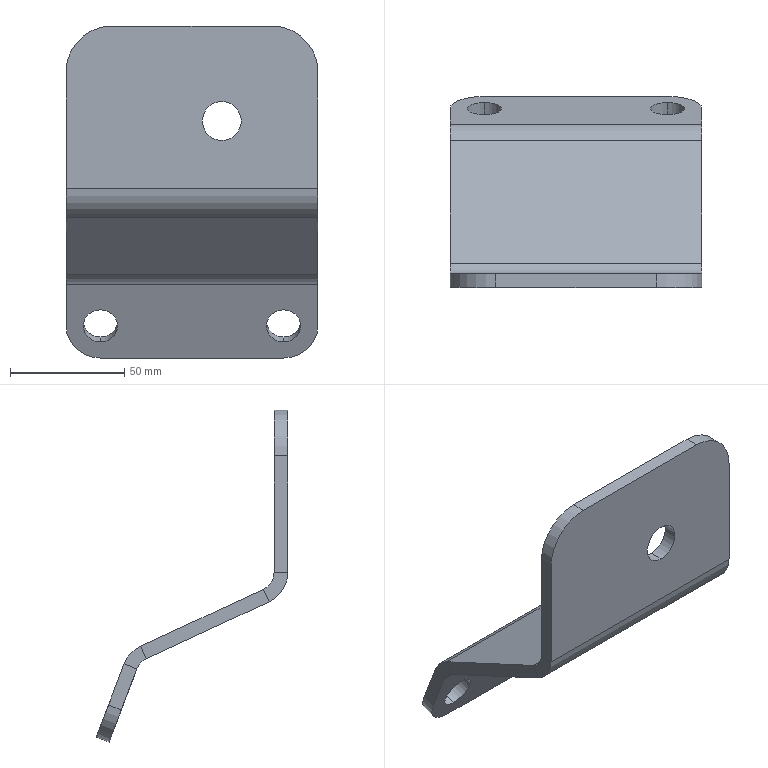Part | SolidWorks | features Fillet 2, ICE 2, FlatPattern 1, SMBaseFlange 1, SheetMetal 1 | 1 solid | 32 faces | box 110 x 83.637 x 145 mm | volume 117261 mm3 | plane 18 | cylinder 14 | commonest cylinder face diameters 15 x4 16 x2 17 x2 28 x2 30 x2 40 x2
STEP:
#1=CARTESIAN_POINT('',(-40.,70.022,-123.973));
#2=VERTEX_POINT('',#1);
#3=CARTESIAN_POINT('',(-40.,75.361,-137.991));
#4=VERTEX_POINT('',#3);
#5=CARTESIAN_POINT('',(-40.,72.691,-130.982));
#6=DIRECTION('',(0.,-0.9345,-0.3559));
#7=DIRECTION('',(0.,-0.3559,0.9345));
#8=AXIS2_PLACEMENT_3D('',#5,#6,#7);
#9=CIRCLE('',#8,7.5);
#10=EDGE_CURVE('',#2,#4,#9,.T.);
#11=ORIENTED_EDGE('',*,*,#10,.T.);
#12=CARTESIAN_POINT('',(-40.,80.968,-135.856));
#13=VERTEX_POINT('',#12);
#14=CARTESIAN_POINT('',(-40.,7.214,-163.946));
#15=DIRECTION('',(0.,0.9345,0.3559));
#16=VECTOR('',#15,1000.);
#17=LINE('',#14,#16);
#18=EDGE_CURVE('',#4,#13,#17,.T.);
#19=ORIENTED_EDGE('',*,*,#18,.T.);
#20=CARTESIAN_POINT('',(-40.,75.629,-121.838));
#21=VERTEX_POINT('',#20);
#22=CARTESIAN_POINT('',(-40.,78.298,-128.847));
#23=DIRECTION('',(0.,0.9345,0.3559));
#24=DIRECTION('',(0.,-0.3559,0.9345));
#25=AXIS2_PLACEMENT_3D('',#22,#23,#24);
#26=CIRCLE('',#25,7.5);
#27=EDGE_CURVE('',#13,#21,#26,.T.);
#28=ORIENTED_EDGE('',*,*,#27,.T.);
#29=CARTESIAN_POINT('',(-40.,1.875,-149.928));
#30=DIRECTION('',(0.,0.9345,0.3559));
#31=VECTOR('',#30,1000.);
#32=LINE('',#29,#31);
#33=EDGE_CURVE('',#2,#21,#32,.T.);
#34=ORIENTED_EDGE('',*,*,#33,.F.);
#35=EDGE_LOOP('',(#11,#19,#28,#34));
#36=FACE_OUTER_BOUND('',#35,.T.);
#37=CARTESIAN_POINT('',(-40.,4.545,-156.937));
#38=DIRECTION('',(0.,0.9345,0.3559));
#39=DIRECTION('',(0.,-0.3559,0.9345));
#40=AXIS2_PLACEMENT_3D('',#37,#38,#39);
#41=CYLINDRICAL_SURFACE('',#40,7.5);
#42=ADVANCED_FACE('',(#36),#41,.F.);
#43=CARTESIAN_POINT('',(40.,70.022,-123.973));
#44=VERTEX_POINT('',#43);
#45=CARTESIAN_POINT('',(40.,75.361,-137.991));
#46=VERTEX_POINT('',#45);
#47=CARTESIAN_POINT('',(40.,72.691,-130.982));
#48=DIRECTION('',(0.,-0.9345,-0.3559));
#49=DIRECTION('',(0.,-0.3559,0.9345));
#50=AXIS2_PLACEMENT_3D('',#47,#48,#49);
#51=CIRCLE('',#50,7.5);
#52=EDGE_CURVE('',#44,#46,#51,.T.);
#53=ORIENTED_EDGE('',*,*,#52,.T.);
#54=CARTESIAN_POINT('',(40.,80.968,-135.856));
#55=VERTEX_POINT('',#54);
#56=CARTESIAN_POINT('',(40.,7.214,-163.946));
#57=DIRECTION('',(0.,0.9345,0.3559));
#58=VECTOR('',#57,1000.);
#59=LINE('',#56,#58);
#60=EDGE_CURVE('',#46,#55,#59,.T.);
#61=ORIENTED_EDGE('',*,*,#60,.T.);
#62=CARTESIAN_POINT('',(40.,75.629,-121.838));
#63=VERTEX_POINT('',#62);
#64=CARTESIAN_POINT('',(40.,78.298,-128.847));
#65=DIRECTION('',(0.,0.9345,0.3559));
#66=DIRECTION('',(0.,-0.3559,0.9345));
#67=AXIS2_PLACEMENT_3D('',#64,#65,#66);
#68=CIRCLE('',#67,7.5);
#69=EDGE_CURVE('',#55,#63,#68,.T.);
#70=ORIENTED_EDGE('',*,*,#69,.T.);
#71=CARTESIAN_POINT('',(40.,1.875,-149.928));
#72=DIRECTION('',(0.,0.9345,0.3559));
#73=VECTOR('',#72,1000.);
#74=LINE('',#71,#73);
#75=EDGE_CURVE('',#44,#63,#74,.T.);
#76=ORIENTED_EDGE('',*,*,#75,.F.);
#77=EDGE_LOOP('',(#53,#61,#70,#76));
#78=FACE_OUTER_BOUND('',#77,.T.);
#79=CARTESIAN_POINT('',(40.,4.545,-156.937));
#80=DIRECTION('',(0.,0.9345,0.3559));
#81=DIRECTION('',(0.,-0.3559,0.9345));
#82=AXIS2_PLACEMENT_3D('',#79,#80,#81);
#83=CYLINDRICAL_SURFACE('',#82,7.5);
#84=ADVANCED_FACE('',(#78),#83,.F.);
#85=CARTESIAN_POINT('',(13.,6.,-33.));
#86=VERTEX_POINT('',#85);
#87=CARTESIAN_POINT('',(13.,6.,-50.));
#88=VERTEX_POINT('',#87);
#89=CARTESIAN_POINT('',(13.,6.,-41.5));
#90=DIRECTION('',(0.,-1.,0.));
#91=DIRECTION('',(0.,0.,1.));
#92=AXIS2_PLACEMENT_3D('',#89,#90,#91);
#93=CIRCLE('',#92,8.5);
#94=EDGE_CURVE('',#86,#88,#93,.T.);
#95=ORIENTED_EDGE('',*,*,#94,.F.);
#96=CARTESIAN_POINT('',(13.,0.,-33.));
#97=VERTEX_POINT('',#96);
#98=CARTESIAN_POINT('',(13.,83.638,-33.));
#99=DIRECTION('',(0.,-1.,0.));
#100=VECTOR('',#99,1000.);
#101=LINE('',#98,#100);
#102=EDGE_CURVE('',#86,#97,#101,.T.);
#103=ORIENTED_EDGE('',*,*,#102,.T.);
#104=CARTESIAN_POINT('',(13.,0.,-50.));
#105=VERTEX_POINT('',#104);
#106=CARTESIAN_POINT('',(13.,0.,-41.5));
#107=DIRECTION('',(0.,-1.,0.));
#108=DIRECTION('',(0.,0.,-1.));
#109=AXIS2_PLACEMENT_3D('',#106,#107,#108);
#110=CIRCLE('',#109,8.5);
#111=EDGE_CURVE('',#97,#105,#110,.T.);
#112=ORIENTED_EDGE('',*,*,#111,.T.);
#113=CARTESIAN_POINT('',(13.,83.638,-50.));
#114=DIRECTION('',(0.,-1.,0.));
#115=VECTOR('',#114,1000.);
#116=LINE('',#113,#115);
#117=EDGE_CURVE('',#88,#105,#116,.T.);
#118=ORIENTED_EDGE('',*,*,#117,.F.);
#119=EDGE_LOOP('',(#95,#103,#112,#118));
#120=FACE_OUTER_BOUND('',#119,.T.);
#121=CARTESIAN_POINT('',(13.,83.638,-41.5));
#122=DIRECTION('',(0.,-1.,0.));
#123=DIRECTION('',(0.,0.,-1.));
#124=AXIS2_PLACEMENT_3D('',#121,#122,#123);
#125=CYLINDRICAL_SURFACE('',#124,8.5);
#126=ADVANCED_FACE('',(#120),#125,.F.);
#127=CARTESIAN_POINT('',(55.,0.,-71.06));
#128=VERTEX_POINT('',#127);
#129=CARTESIAN_POINT('',(55.,6.,-71.06));
#130=VERTEX_POINT('',#129);
#131=CARTESIAN_POINT('',(55.,0.,-71.06));
#132=DIRECTION('',(0.,1.,0.));
#133=VECTOR('',#132,1000.);
#134=LINE('',#131,#133);
#135=EDGE_CURVE('',#128,#130,#134,.T.);
#136=ORIENTED_EDGE('',*,*,#135,.F.);
#137=CARTESIAN_POINT('',(55.,8.111,-83.761));
#138=VERTEX_POINT('',#137);
#139=CARTESIAN_POINT('',(55.,14.,-71.06));
#140=DIRECTION('',(1.,0.,0.));
#141=DIRECTION('',(0.,0.,1.));
#142=AXIS2_PLACEMENT_3D('',#139,#140,#141);
#143=CIRCLE('',#142,14.);
#144=EDGE_CURVE('',#128,#138,#143,.T.);
#145=ORIENTED_EDGE('',*,*,#144,.T.);
#146=CARTESIAN_POINT('',(55.,10.635,-78.317));
#147=VERTEX_POINT('',#146);
#148=CARTESIAN_POINT('',(55.,10.635,-78.317));
#149=DIRECTION('',(0.,-0.4207,-0.9072));
#150=VECTOR('',#149,1000.);
#151=LINE('',#148,#150);
#152=EDGE_CURVE('',#147,#138,#151,.T.);
#153=ORIENTED_EDGE('',*,*,#152,.F.);
#154=CARTESIAN_POINT('',(55.,14.,-71.06));
#155=DIRECTION('',(1.,0.,0.));
#156=DIRECTION('',(0.,0.,-1.));
#157=AXIS2_PLACEMENT_3D('',#154,#155,#156);
#158=CIRCLE('',#157,8.);
#159=EDGE_CURVE('',#130,#147,#158,.T.);
#160=ORIENTED_EDGE('',*,*,#159,.F.);
#161=EDGE_LOOP('',(#136,#145,#153,#160));
#162=FACE_OUTER_BOUND('',#161,.T.);
#163=CARTESIAN_POINT('',(55.,0.,-71.06));
#164=DIRECTION('',(1.,0.,0.));
#165=DIRECTION('',(0.,0.,-1.));
#166=AXIS2_PLACEMENT_3D('',#163,#164,#165);
#167=PLANE('',#166);
#168=ADVANCED_FACE('',(#162),#167,.T.);
#169=CARTESIAN_POINT('',(55.,6.,-20.));
#170=VERTEX_POINT('',#169);
#171=CARTESIAN_POINT('',(55.,6.,0.));
#172=DIRECTION('',(0.,0.,-1.));
#173=VECTOR('',#172,1000.);
#174=LINE('',#171,#173);
#175=EDGE_CURVE('',#170,#130,#174,.T.);
#176=ORIENTED_EDGE('',*,*,#175,.F.);
#177=CARTESIAN_POINT('',(55.,0.,-20.));
#178=VERTEX_POINT('',#177);
#179=CARTESIAN_POINT('',(55.,10.635,-20.));
#180=DIRECTION('',(0.,-1.,0.));
#181=VECTOR('',#180,1000.);
#182=LINE('',#179,#181);
#183=EDGE_CURVE('',#170,#178,#182,.T.);
#184=ORIENTED_EDGE('',*,*,#183,.T.);
#185=CARTESIAN_POINT('',(55.,0.,0.));
#186=DIRECTION('',(0.,0.,-1.));
#187=VECTOR('',#186,1000.);
#188=LINE('',#185,#187);
#189=EDGE_CURVE('',#178,#128,#188,.T.);
#190=ORIENTED_EDGE('',*,*,#189,.T.);
#191=ORIENTED_EDGE('',*,*,#135,.T.);
#192=EDGE_LOOP('',(#176,#184,#190,#191));
#193=FACE_OUTER_BOUND('',#192,.T.);
#194=CARTESIAN_POINT('',(55.,10.635,-78.317));
#195=DIRECTION('',(1.,0.,0.));
#196=DIRECTION('',(0.,0.,-1.));
#197=AXIS2_PLACEMENT_3D('',#194,#195,#196);
#198=PLANE('',#197);
#199=ADVANCED_FACE('',(#193),#198,.T.);
#200=CARTESIAN_POINT('',(-55.,8.111,-83.761));
#201=VERTEX_POINT('',#200);
#202=CARTESIAN_POINT('',(-55.,10.635,-78.317));
#203=VERTEX_POINT('',#202);
#204=CARTESIAN_POINT('',(-55.,8.111,-83.761));
#205=DIRECTION('',(0.,0.4207,0.9072));
#206=VECTOR('',#205,1000.);
#207=LINE('',#204,#206);
#208=EDGE_CURVE('',#201,#203,#207,.T.);
#209=ORIENTED_EDGE('',*,*,#208,.F.);
#210=CARTESIAN_POINT('',(-55.,0.,-71.06));
#211=VERTEX_POINT('',#210);
#212=CARTESIAN_POINT('',(-55.,14.,-71.06));
#213=DIRECTION('',(1.,0.,0.));
#214=DIRECTION('',(0.,0.,1.));
#215=AXIS2_PLACEMENT_3D('',#212,#213,#214);
#216=CIRCLE('',#215,14.);
#217=EDGE_CURVE('',#211,#201,#216,.T.);
#218=ORIENTED_EDGE('',*,*,#217,.F.);
#219=CARTESIAN_POINT('',(-55.,6.,-71.06));
#220=VERTEX_POINT('',#219);
#221=CARTESIAN_POINT('',(-55.,6.,-71.06));
#222=DIRECTION('',(0.,-1.,0.));
#223=VECTOR('',#222,1000.);
#224=LINE('',#221,#223);
#225=EDGE_CURVE('',#220,#211,#224,.T.);
#226=ORIENTED_EDGE('',*,*,#225,.F.);
#227=CARTESIAN_POINT('',(-55.,14.,-71.06));
#228=DIRECTION('',(1.,0.,0.));
#229=DIRECTION('',(0.,0.,-1.));
#230=AXIS2_PLACEMENT_3D('',#227,#228,#229);
#231=CIRCLE('',#230,8.);
#232=EDGE_CURVE('',#220,#203,#231,.T.);
#233=ORIENTED_EDGE('',*,*,#232,.T.);
#234=EDGE_LOOP('',(#209,#218,#226,#233));
#235=FACE_OUTER_BOUND('',#234,.T.);
#236=CARTESIAN_POINT('',(-55.,8.111,-83.761));
#237=DIRECTION('',(-1.,0.,0.));
#238=DIRECTION('',(0.,0.,1.));
#239=AXIS2_PLACEMENT_3D('',#236,#237,#238);
#240=PLANE('',#239);
#241=ADVANCED_FACE('',(#235),#240,.T.);
#242=CARTESIAN_POINT('',(-55.,61.747,-108.631));
#243=VERTEX_POINT('',#242);
#244=CARTESIAN_POINT('',(-55.,0.,-80.));
#245=DIRECTION('',(0.,0.9072,-0.4207));
#246=VECTOR('',#245,1000.);
#247=LINE('',#244,#246);
#248=EDGE_CURVE('',#201,#243,#247,.T.);
#249=ORIENTED_EDGE('',*,*,#248,.F.);
#250=ORIENTED_EDGE('',*,*,#208,.T.);
#251=CARTESIAN_POINT('',(-55.,64.271,-103.188));
#252=VERTEX_POINT('',#251);
#253=CARTESIAN_POINT('',(-55.,2.524,-74.557));
#254=DIRECTION('',(0.,0.9072,-0.4207));
#255=VECTOR('',#254,1000.);
#256=LINE('',#253,#255);
#257=EDGE_CURVE('',#203,#252,#256,.T.);
#258=ORIENTED_EDGE('',*,*,#257,.T.);
#259=CARTESIAN_POINT('',(-55.,64.271,-103.188));
#260=DIRECTION('',(0.,-0.4207,-0.9072));
#261=VECTOR('',#260,1000.);
#262=LINE('',#259,#261);
#263=EDGE_CURVE('',#252,#243,#262,.T.);
#264=ORIENTED_EDGE('',*,*,#263,.T.);
#265=EDGE_LOOP('',(#249,#250,#258,#264));
#266=FACE_OUTER_BOUND('',#265,.T.);
#267=CARTESIAN_POINT('',(-55.,6.,-71.06));
#268=DIRECTION('',(-1.,0.,0.));
#269=DIRECTION('',(0.,0.,1.));
#270=AXIS2_PLACEMENT_3D('',#267,#268,#269);
#271=PLANE('',#270);
#272=ADVANCED_FACE('',(#266),#271,.T.);
#273=CARTESIAN_POINT('',(55.,61.747,-108.631));
#274=VERTEX_POINT('',#273);
#275=CARTESIAN_POINT('',(55.,64.271,-103.188));
#276=VERTEX_POINT('',#275);
#277=CARTESIAN_POINT('',(55.,61.747,-108.631));
#278=DIRECTION('',(0.,0.4207,0.9072));
#279=VECTOR('',#278,1000.);
#280=LINE('',#277,#279);
#281=EDGE_CURVE('',#274,#276,#280,.T.);
#282=ORIENTED_EDGE('',*,*,#281,.F.);
#283=CARTESIAN_POINT('',(55.,65.858,-113.041));
#284=VERTEX_POINT('',#283);
#285=CARTESIAN_POINT('',(55.,58.382,-115.889));
#286=DIRECTION('',(-1.,0.,0.));
#287=DIRECTION('',(0.,0.,-1.));
#288=AXIS2_PLACEMENT_3D('',#285,#286,#287);
#289=CIRCLE('',#288,8.);
#290=EDGE_CURVE('',#274,#284,#289,.T.);
#291=ORIENTED_EDGE('',*,*,#290,.T.);
#292=CARTESIAN_POINT('',(55.,71.465,-110.906));
#293=VERTEX_POINT('',#292);
#294=CARTESIAN_POINT('',(55.,71.465,-110.906));
#295=DIRECTION('',(0.,-0.9345,-0.3559));
#296=VECTOR('',#295,1000.);
#297=LINE('',#294,#296);
#298=EDGE_CURVE('',#293,#284,#297,.T.);
#299=ORIENTED_EDGE('',*,*,#298,.F.);
#300=CARTESIAN_POINT('',(55.,58.382,-115.889));
#301=DIRECTION('',(-1.,0.,0.));
#302=DIRECTION('',(0.,0.,-1.));
#303=AXIS2_PLACEMENT_3D('',#300,#301,#302);
#304=CIRCLE('',#303,14.);
#305=EDGE_CURVE('',#276,#293,#304,.T.);
#306=ORIENTED_EDGE('',*,*,#305,.F.);
#307=EDGE_LOOP('',(#282,#291,#299,#306));
#308=FACE_OUTER_BOUND('',#307,.T.);
#309=CARTESIAN_POINT('',(55.,61.747,-108.631));
#310=DIRECTION('',(1.,0.,0.));
#311=DIRECTION('',(0.,0.,-1.));
#312=AXIS2_PLACEMENT_3D('',#309,#310,#311);
#313=PLANE('',#312);
#314=ADVANCED_FACE('',(#308),#313,.T.);
#315=CARTESIAN_POINT('',(55.,0.,-80.));
#316=DIRECTION('',(0.,0.9072,-0.4207));
#317=VECTOR('',#316,1000.);
#318=LINE('',#315,#317);
#319=EDGE_CURVE('',#138,#274,#318,.T.);
#320=ORIENTED_EDGE('',*,*,#319,.T.);
#321=ORIENTED_EDGE('',*,*,#281,.T.);
#322=CARTESIAN_POINT('',(55.,2.524,-74.557));
#323=DIRECTION('',(0.,0.9072,-0.4207));
#324=VECTOR('',#323,1000.);
#325=LINE('',#322,#324);
#326=EDGE_CURVE('',#147,#276,#325,.T.);
#327=ORIENTED_EDGE('',*,*,#326,.F.);
#328=ORIENTED_EDGE('',*,*,#152,.T.);
#329=EDGE_LOOP('',(#320,#321,#327,#328));
#330=FACE_OUTER_BOUND('',#329,.T.);
#331=CARTESIAN_POINT('',(55.,71.465,-110.906));
#332=DIRECTION('',(1.,0.,0.));
#333=DIRECTION('',(0.,0.,-1.));
#334=AXIS2_PLACEMENT_3D('',#331,#332,#333);
#335=PLANE('',#334);
#336=ADVANCED_FACE('',(#330),#335,.T.);
#337=CARTESIAN_POINT('',(-55.,65.858,-113.041));
#338=VERTEX_POINT('',#337);
#339=CARTESIAN_POINT('',(-55.,71.465,-110.906));
#340=VERTEX_POINT('',#339);
#341=CARTESIAN_POINT('',(-55.,65.858,-113.041));
#342=DIRECTION('',(0.,0.9345,0.3559));
#343=VECTOR('',#342,1000.);
#344=LINE('',#341,#343);
#345=EDGE_CURVE('',#338,#340,#344,.T.);
#346=ORIENTED_EDGE('',*,*,#345,.F.);
#347=CARTESIAN_POINT('',(-55.,58.382,-115.889));
#348=DIRECTION('',(-1.,0.,0.));
#349=DIRECTION('',(0.,0.,-1.));
#350=AXIS2_PLACEMENT_3D('',#347,#348,#349);
#351=CIRCLE('',#350,8.);
#352=EDGE_CURVE('',#243,#338,#351,.T.);
#353=ORIENTED_EDGE('',*,*,#352,.F.);
#354=ORIENTED_EDGE('',*,*,#263,.F.);
#355=CARTESIAN_POINT('',(-55.,58.382,-115.889));
#356=DIRECTION('',(-1.,0.,0.));
#357=DIRECTION('',(0.,0.,-1.));
#358=AXIS2_PLACEMENT_3D('',#355,#356,#357);
#359=CIRCLE('',#358,14.);
#360=EDGE_CURVE('',#252,#340,#359,.T.);
#361=ORIENTED_EDGE('',*,*,#360,.T.);
#362=EDGE_LOOP('',(#346,#353,#354,#361));
#363=FACE_OUTER_BOUND('',#362,.T.);
#364=CARTESIAN_POINT('',(-55.,65.858,-113.041));
#365=DIRECTION('',(-1.,0.,0.));
#366=DIRECTION('',(0.,0.,1.));
#367=AXIS2_PLACEMENT_3D('',#364,#365,#366);
#368=PLANE('',#367);
#369=ADVANCED_FACE('',(#363),#368,.T.);
#370=CARTESIAN_POINT('',(-55.,78.298,-128.847));
#371=VERTEX_POINT('',#370);
#372=CARTESIAN_POINT('',(-55.,70.307,-107.864));
#373=DIRECTION('',(0.,0.3559,-0.9345));
#374=VECTOR('',#373,1000.);
#375=LINE('',#372,#374);
#376=EDGE_CURVE('',#340,#371,#375,.T.);
#377=ORIENTED_EDGE('',*,*,#376,.T.);
#378=CARTESIAN_POINT('',(-55.,72.691,-130.982));
#379=VERTEX_POINT('',#378);
#380=CARTESIAN_POINT('',(-55.,74.583,-130.262));
#381=DIRECTION('',(0.,-0.9345,-0.3559));
#382=VECTOR('',#381,1000.);
#383=LINE('',#380,#382);
#384=EDGE_CURVE('',#371,#379,#383,.T.);
#385=ORIENTED_EDGE('',*,*,#384,.T.);
#386=CARTESIAN_POINT('',(-55.,64.7,-110.));
#387=DIRECTION('',(0.,0.3559,-0.9345));
#388=VECTOR('',#387,1000.);
#389=LINE('',#386,#388);
#390=EDGE_CURVE('',#338,#379,#389,.T.);
#391=ORIENTED_EDGE('',*,*,#390,.F.);
#392=ORIENTED_EDGE('',*,*,#345,.T.);
#393=EDGE_LOOP('',(#377,#385,#391,#392));
#394=FACE_OUTER_BOUND('',#393,.T.);
#395=CARTESIAN_POINT('',(-55.,64.271,-103.188));
#396=DIRECTION('',(-1.,0.,0.));
#397=DIRECTION('',(0.,0.,1.));
#398=AXIS2_PLACEMENT_3D('',#395,#396,#397);
#399=PLANE('',#398);
#400=ADVANCED_FACE('',(#394),#399,.T.);
#401=ORIENTED_EDGE('',*,*,#10,.F.);
#402=CARTESIAN_POINT('',(-40.,72.691,-130.982));
#403=DIRECTION('',(0.,-0.9345,-0.3559));
#404=DIRECTION('',(0.,-0.3559,0.9345));
#405=AXIS2_PLACEMENT_3D('',#402,#403,#404);
#406=CIRCLE('',#405,7.5);
#407=EDGE_CURVE('',#4,#2,#406,.T.);
#408=ORIENTED_EDGE('',*,*,#407,.F.);
#409=EDGE_LOOP('',(#401,#408));
#410=FACE_BOUND('',#409,.T.);
#411=ORIENTED_EDGE('',*,*,#52,.F.);
#412=CARTESIAN_POINT('',(40.,72.691,-130.982));
#413=DIRECTION('',(0.,-0.9345,-0.3559));
#414=DIRECTION('',(0.,-0.3559,0.9345));
#415=AXIS2_PLACEMENT_3D('',#412,#413,#414);
#416=CIRCLE('',#415,7.5);
#417=EDGE_CURVE('',#46,#44,#416,.T.);
#418=ORIENTED_EDGE('',*,*,#417,.F.);
#419=EDGE_LOOP('',(#411,#418));
#420=FACE_BOUND('',#419,.T.);
#421=ORIENTED_EDGE('',*,*,#390,.T.);
#422=CARTESIAN_POINT('',(-40.,78.03,-145.));
#423=VERTEX_POINT('',#422);
#424=CARTESIAN_POINT('',(-40.,72.691,-130.982));
#425=DIRECTION('',(0.,-0.9345,-0.3559));
#426=DIRECTION('',(0.,-0.3559,0.9345));
#427=AXIS2_PLACEMENT_3D('',#424,#425,#426);
#428=CIRCLE('',#427,15.);
#429=EDGE_CURVE('',#379,#423,#428,.T.);
#430=ORIENTED_EDGE('',*,*,#429,.T.);
#431=CARTESIAN_POINT('',(40.,78.03,-145.));
#432=VERTEX_POINT('',#431);
#433=CARTESIAN_POINT('',(55.,78.03,-145.));
#434=DIRECTION('',(-1.,0.,0.));
#435=VECTOR('',#434,1000.);
#436=LINE('',#433,#435);
#437=EDGE_CURVE('',#432,#423,#436,.T.);
#438=ORIENTED_EDGE('',*,*,#437,.F.);
#439=CARTESIAN_POINT('',(55.,72.691,-130.982));
#440=VERTEX_POINT('',#439);
#441=CARTESIAN_POINT('',(40.,72.691,-130.982));
#442=DIRECTION('',(0.,-0.9345,-0.3559));
#443=DIRECTION('',(0.,-0.3559,0.9345));
#444=AXIS2_PLACEMENT_3D('',#441,#442,#443);
#445=CIRCLE('',#444,15.);
#446=EDGE_CURVE('',#432,#440,#445,.T.);
#447=ORIENTED_EDGE('',*,*,#446,.T.);
#448=CARTESIAN_POINT('',(55.,64.7,-110.));
#449=DIRECTION('',(0.,0.3559,-0.9345));
#450=VECTOR('',#449,1000.);
#451=LINE('',#448,#450);
#452=EDGE_CURVE('',#284,#440,#451,.T.);
#453=ORIENTED_EDGE('',*,*,#452,.F.);
#454=CARTESIAN_POINT('',(55.,65.858,-113.041));
#455=DIRECTION('',(-1.,0.,0.));
#456=VECTOR('',#455,1000.);
#457=LINE('',#454,#456);
#458=EDGE_CURVE('',#284,#338,#457,.T.);
#459=ORIENTED_EDGE('',*,*,#458,.T.);
#460=EDGE_LOOP('',(#421,#430,#438,#447,#453,#459));
#461=FACE_OUTER_BOUND('',#460,.T.);
#462=CARTESIAN_POINT('',(55.,64.7,-110.));
#463=DIRECTION('',(0.,0.9345,0.3559));
#464=DIRECTION('',(0.,-0.3559,0.9345));
#465=AXIS2_PLACEMENT_3D('',#462,#463,#464);
#466=PLANE('',#465);
#467=ADVANCED_FACE('',(#410,#420,#461),#466,.F.);
#468=ORIENTED_EDGE('',*,*,#437,.T.);
#469=CARTESIAN_POINT('',(-40.,83.637,-142.864));
#470=VERTEX_POINT('',#469);
#471=CARTESIAN_POINT('',(-40.,83.637,-142.864));
#472=DIRECTION('',(0.,0.9345,0.3559));
#473=VECTOR('',#472,1000.);
#474=LINE('',#471,#473);
#475=EDGE_CURVE('',#423,#470,#474,.T.);
#476=ORIENTED_EDGE('',*,*,#475,.T.);
#477=CARTESIAN_POINT('',(40.,83.637,-142.864));
#478=VERTEX_POINT('',#477);
#479=CARTESIAN_POINT('',(55.,83.637,-142.864));
#480=DIRECTION('',(-1.,0.,0.));
#481=VECTOR('',#480,1000.);
#482=LINE('',#479,#481);
#483=EDGE_CURVE('',#478,#470,#482,.T.);
#484=ORIENTED_EDGE('',*,*,#483,.F.);
#485=CARTESIAN_POINT('',(40.,83.637,-142.864));
#486=DIRECTION('',(0.,-0.9345,-0.3559));
#487=VECTOR('',#486,1000.);
#488=LINE('',#485,#487);
#489=EDGE_CURVE('',#478,#432,#488,.T.);
#490=ORIENTED_EDGE('',*,*,#489,.T.);
#491=EDGE_LOOP('',(#468,#476,#484,#490));
#492=FACE_OUTER_BOUND('',#491,.T.);
#493=CARTESIAN_POINT('',(55.,83.637,-142.864));
#494=DIRECTION('',(0.,0.3559,-0.9345));
#495=DIRECTION('',(0.,0.9345,0.3559));
#496=AXIS2_PLACEMENT_3D('',#493,#494,#495);
#497=PLANE('',#496);
#498=ADVANCED_FACE('',(#492),#497,.T.);
#499=CARTESIAN_POINT('',(-40.,78.298,-128.847));
#500=DIRECTION('',(0.,0.9345,0.3559));
#501=DIRECTION('',(0.,-0.3559,0.9345));
#502=AXIS2_PLACEMENT_3D('',#499,#500,#501);
#503=CIRCLE('',#502,7.5);
#504=EDGE_CURVE('',#21,#13,#503,.T.);
#505=ORIENTED_EDGE('',*,*,#504,.F.);
#506=ORIENTED_EDGE('',*,*,#27,.F.);
#507=EDGE_LOOP('',(#505,#506));
#508=FACE_BOUND('',#507,.T.);
#509=CARTESIAN_POINT('',(40.,78.298,-128.847));
#510=DIRECTION('',(0.,0.9345,0.3559));
#511=DIRECTION('',(0.,-0.3559,0.9345));
#512=AXIS2_PLACEMENT_3D('',#509,#510,#511);
#513=CIRCLE('',#512,7.5);
#514=EDGE_CURVE('',#63,#55,#513,.T.);
#515=ORIENTED_EDGE('',*,*,#514,.F.);
#516=ORIENTED_EDGE('',*,*,#69,.F.);
#517=EDGE_LOOP('',(#515,#516));
#518=FACE_BOUND('',#517,.T.);
#519=ORIENTED_EDGE('',*,*,#483,.T.);
#520=CARTESIAN_POINT('',(-40.,78.298,-128.847));
#521=DIRECTION('',(0.,0.9345,0.3559));
#522=DIRECTION('',(0.,-0.3559,0.9345));
#523=AXIS2_PLACEMENT_3D('',#520,#521,#522);
#524=CIRCLE('',#523,15.);
#525=EDGE_CURVE('',#470,#371,#524,.T.);
#526=ORIENTED_EDGE('',*,*,#525,.T.);
#527=ORIENTED_EDGE('',*,*,#376,.F.);
#528=CARTESIAN_POINT('',(55.,71.465,-110.906));
#529=DIRECTION('',(-1.,0.,0.));
#530=VECTOR('',#529,1000.);
#531=LINE('',#528,#530);
#532=EDGE_CURVE('',#293,#340,#531,.T.);
#533=ORIENTED_EDGE('',*,*,#532,.F.);
#534=CARTESIAN_POINT('',(55.,78.298,-128.847));
#535=VERTEX_POINT('',#534);
#536=CARTESIAN_POINT('',(55.,70.307,-107.864));
#537=DIRECTION('',(0.,0.3559,-0.9345));
#538=VECTOR('',#537,1000.);
#539=LINE('',#536,#538);
#540=EDGE_CURVE('',#293,#535,#539,.T.);
#541=ORIENTED_EDGE('',*,*,#540,.T.);
#542=CARTESIAN_POINT('',(40.,78.298,-128.847));
#543=DIRECTION('',(0.,0.9345,0.3559));
#544=DIRECTION('',(0.,-0.3559,0.9345));
#545=AXIS2_PLACEMENT_3D('',#542,#543,#544);
#546=CIRCLE('',#545,15.);
#547=EDGE_CURVE('',#535,#478,#546,.T.);
#548=ORIENTED_EDGE('',*,*,#547,.T.);
#549=EDGE_LOOP('',(#519,#526,#527,#533,#541,#548));
#550=FACE_OUTER_BOUND('',#549,.T.);
#551=CARTESIAN_POINT('',(55.,70.307,-107.864));
#552=DIRECTION('',(0.,0.9345,0.3559));
#553=DIRECTION('',(0.,-0.3559,0.9345));
#554=AXIS2_PLACEMENT_3D('',#551,#552,#553);
#555=PLANE('',#554);
#556=ADVANCED_FACE('',(#508,#518,#550),#555,.T.);
#557=ORIENTED_EDGE('',*,*,#360,.F.);
#558=CARTESIAN_POINT('',(55.,64.271,-103.188));
#559=DIRECTION('',(-1.,0.,0.));
#560=VECTOR('',#559,1000.);
#561=LINE('',#558,#560);
#562=EDGE_CURVE('',#276,#252,#561,.T.);
#563=ORIENTED_EDGE('',*,*,#562,.F.);
#564=ORIENTED_EDGE('',*,*,#305,.T.);
#565=ORIENTED_EDGE('',*,*,#532,.T.);
#566=EDGE_LOOP('',(#557,#563,#564,#565));
#567=FACE_OUTER_BOUND('',#566,.T.);
#568=CARTESIAN_POINT('',(55.,58.382,-115.889));
#569=DIRECTION('',(-1.,0.,0.));
#570=DIRECTION('',(0.,0.,1.));
#571=AXIS2_PLACEMENT_3D('',#568,#569,#570);
#572=CYLINDRICAL_SURFACE('',#571,14.);
#573=ADVANCED_FACE('',(#567),#572,.T.);
#574=ORIENTED_EDGE('',*,*,#257,.F.);
#575=CARTESIAN_POINT('',(55.,10.635,-78.317));
#576=DIRECTION('',(-1.,0.,0.));
#577=VECTOR('',#576,1000.);
#578=LINE('',#575,#577);
#579=EDGE_CURVE('',#147,#203,#578,.T.);
#580=ORIENTED_EDGE('',*,*,#579,.F.);
#581=ORIENTED_EDGE('',*,*,#326,.T.);
#582=ORIENTED_EDGE('',*,*,#562,.T.);
#583=EDGE_LOOP('',(#574,#580,#581,#582));
#584=FACE_OUTER_BOUND('',#583,.T.);
#585=CARTESIAN_POINT('',(55.,2.524,-74.557));
#586=DIRECTION('',(0.,0.4207,0.9072));
#587=DIRECTION('',(0.,-0.9072,0.4207));
#588=AXIS2_PLACEMENT_3D('',#585,#586,#587);
#589=PLANE('',#588);
#590=ADVANCED_FACE('',(#584),#589,.T.);
#591=ORIENTED_EDGE('',*,*,#232,.F.);
#592=CARTESIAN_POINT('',(55.,6.,-71.06));
#593=DIRECTION('',(-1.,0.,0.));
#594=VECTOR('',#593,1000.);
#595=LINE('',#592,#594);
#596=EDGE_CURVE('',#130,#220,#595,.T.);
#597=ORIENTED_EDGE('',*,*,#596,.F.);
#598=ORIENTED_EDGE('',*,*,#159,.T.);
#599=ORIENTED_EDGE('',*,*,#579,.T.);
#600=EDGE_LOOP('',(#591,#597,#598,#599));
#601=FACE_OUTER_BOUND('',#600,.T.);
#602=CARTESIAN_POINT('',(55.,14.,-71.06));
#603=DIRECTION('',(-1.,0.,0.));
#604=DIRECTION('',(0.,0.,1.));
#605=AXIS2_PLACEMENT_3D('',#602,#603,#604);
#606=CYLINDRICAL_SURFACE('',#605,8.);
#607=ADVANCED_FACE('',(#601),#606,.F.);
#608=CARTESIAN_POINT('',(13.,6.,-41.5));
#609=DIRECTION('',(0.,-1.,0.));
#610=DIRECTION('',(0.,0.,1.));
#611=AXIS2_PLACEMENT_3D('',#608,#609,#610);
#612=CIRCLE('',#611,8.5);
#613=EDGE_CURVE('',#88,#86,#612,.T.);
#614=ORIENTED_EDGE('',*,*,#613,.T.);
#615=ORIENTED_EDGE('',*,*,#94,.T.);
#616=EDGE_LOOP('',(#614,#615));
#617=FACE_BOUND('',#616,.T.);
#618=CARTESIAN_POINT('',(35.,6.,0.));
#619=VERTEX_POINT('',#618);
#620=CARTESIAN_POINT('',(-35.,6.,0.));
#621=VERTEX_POINT('',#620);
#622=CARTESIAN_POINT('',(55.,6.,0.));
#623=DIRECTION('',(-1.,0.,0.));
#624=VECTOR('',#623,1000.);
#625=LINE('',#622,#624);
#626=EDGE_CURVE('',#619,#621,#625,.T.);
#627=ORIENTED_EDGE('',*,*,#626,.F.);
#628=CARTESIAN_POINT('',(35.,6.,-20.));
#629=DIRECTION('',(0.,1.,0.));
#630=DIRECTION('',(0.,0.,1.));
#631=AXIS2_PLACEMENT_3D('',#628,#629,#630);
#632=CIRCLE('',#631,20.);
#633=EDGE_CURVE('',#619,#170,#632,.T.);
#634=ORIENTED_EDGE('',*,*,#633,.T.);
#635=ORIENTED_EDGE('',*,*,#175,.T.);
#636=ORIENTED_EDGE('',*,*,#596,.T.);
#637=CARTESIAN_POINT('',(-55.,6.,-20.));
#638=VERTEX_POINT('',#637);
#639=CARTESIAN_POINT('',(-55.,6.,0.));
#640=DIRECTION('',(0.,0.,-1.));
#641=VECTOR('',#640,1000.);
#642=LINE('',#639,#641);
#643=EDGE_CURVE('',#638,#220,#642,.T.);
#644=ORIENTED_EDGE('',*,*,#643,.F.);
#645=CARTESIAN_POINT('',(-35.,6.,-20.));
#646=DIRECTION('',(0.,1.,0.));
#647=DIRECTION('',(0.,0.,1.));
#648=AXIS2_PLACEMENT_3D('',#645,#646,#647);
#649=CIRCLE('',#648,20.);
#650=EDGE_CURVE('',#638,#621,#649,.T.);
#651=ORIENTED_EDGE('',*,*,#650,.T.);
#652=EDGE_LOOP('',(#627,#634,#635,#636,#644,#651));
#653=FACE_OUTER_BOUND('',#652,.T.);
#654=CARTESIAN_POINT('',(55.,6.,0.));
#655=DIRECTION('',(0.,1.,0.));
#656=DIRECTION('',(0.,0.,1.));
#657=AXIS2_PLACEMENT_3D('',#654,#655,#656);
#658=PLANE('',#657);
#659=ADVANCED_FACE('',(#617,#653),#658,.T.);
#660=CARTESIAN_POINT('',(35.,0.,0.));
#661=VERTEX_POINT('',#660);
#662=CARTESIAN_POINT('',(-35.,0.,0.));
#663=VERTEX_POINT('',#662);
#664=CARTESIAN_POINT('',(55.,0.,0.));
#665=DIRECTION('',(-1.,0.,0.));
#666=VECTOR('',#665,1000.);
#667=LINE('',#664,#666);
#668=EDGE_CURVE('',#661,#663,#667,.T.);
#669=ORIENTED_EDGE('',*,*,#668,.F.);
#670=CARTESIAN_POINT('',(35.,0.,0.));
#671=DIRECTION('',(0.,1.,0.));
#672=VECTOR('',#671,1000.);
#673=LINE('',#670,#672);
#674=EDGE_CURVE('',#661,#619,#673,.T.);
#675=ORIENTED_EDGE('',*,*,#674,.T.);
#676=ORIENTED_EDGE('',*,*,#626,.T.);
#677=CARTESIAN_POINT('',(-35.,0.,0.));
#678=DIRECTION('',(0.,-1.,0.));
#679=VECTOR('',#678,1000.);
#680=LINE('',#677,#679);
#681=EDGE_CURVE('',#621,#663,#680,.T.);
#682=ORIENTED_EDGE('',*,*,#681,.T.);
#683=EDGE_LOOP('',(#669,#675,#676,#682));
#684=FACE_OUTER_BOUND('',#683,.T.);
#685=CARTESIAN_POINT('',(55.,0.,0.));
#686=DIRECTION('',(0.,0.,1.));
#687=DIRECTION('',(1.,0.,0.));
#688=AXIS2_PLACEMENT_3D('',#685,#686,#687);
#689=PLANE('',#688);
#690=ADVANCED_FACE('',(#684),#689,.T.);
#691=CARTESIAN_POINT('',(13.,0.,-41.5));
#692=DIRECTION('',(0.,-1.,0.));
#693=DIRECTION('',(0.,0.,-1.));
#694=AXIS2_PLACEMENT_3D('',#691,#692,#693);
#695=CIRCLE('',#694,8.5);
#696=EDGE_CURVE('',#105,#97,#695,.T.);
#697=ORIENTED_EDGE('',*,*,#696,.F.);
#698=ORIENTED_EDGE('',*,*,#111,.F.);
#699=EDGE_LOOP('',(#697,#698));
#700=FACE_BOUND('',#699,.T.);
#701=ORIENTED_EDGE('',*,*,#189,.F.);
#702=CARTESIAN_POINT('',(35.,0.,-20.));
#703=DIRECTION('',(0.,-1.,0.));
#704=DIRECTION('',(0.,0.,1.));
#705=AXIS2_PLACEMENT_3D('',#702,#703,#704);
#706=CIRCLE('',#705,20.);
#707=EDGE_CURVE('',#178,#661,#706,.T.);
#708=ORIENTED_EDGE('',*,*,#707,.T.);
#709=ORIENTED_EDGE('',*,*,#668,.T.);
#710=CARTESIAN_POINT('',(-55.,0.,-20.));
#711=VERTEX_POINT('',#710);
#712=CARTESIAN_POINT('',(-35.,0.,-20.));
#713=DIRECTION('',(0.,-1.,0.));
#714=DIRECTION('',(0.,0.,1.));
#715=AXIS2_PLACEMENT_3D('',#712,#713,#714);
#716=CIRCLE('',#715,20.);
#717=EDGE_CURVE('',#663,#711,#716,.T.);
#718=ORIENTED_EDGE('',*,*,#717,.T.);
#719=CARTESIAN_POINT('',(-55.,0.,0.));
#720=DIRECTION('',(0.,0.,-1.));
#721=VECTOR('',#720,1000.);
#722=LINE('',#719,#721);
#723=EDGE_CURVE('',#711,#211,#722,.T.);
#724=ORIENTED_EDGE('',*,*,#723,.T.);
#725=CARTESIAN_POINT('',(55.,0.,-71.06));
#726=DIRECTION('',(-1.,0.,0.));
#727=VECTOR('',#726,1000.);
#728=LINE('',#725,#727);
#729=EDGE_CURVE('',#128,#211,#728,.T.);
#730=ORIENTED_EDGE('',*,*,#729,.F.);
#731=EDGE_LOOP('',(#701,#708,#709,#718,#724,#730));
#732=FACE_OUTER_BOUND('',#731,.T.);
#733=CARTESIAN_POINT('',(55.,0.,0.));
#734=DIRECTION('',(0.,1.,0.));
#735=DIRECTION('',(0.,0.,1.));
#736=AXIS2_PLACEMENT_3D('',#733,#734,#735);
#737=PLANE('',#736);
#738=ADVANCED_FACE('',(#700,#732),#737,.F.);
#739=ORIENTED_EDGE('',*,*,#217,.T.);
#740=CARTESIAN_POINT('',(55.,8.111,-83.761));
#741=DIRECTION('',(-1.,0.,0.));
#742=VECTOR('',#741,1000.);
#743=LINE('',#740,#742);
#744=EDGE_CURVE('',#138,#201,#743,.T.);
#745=ORIENTED_EDGE('',*,*,#744,.F.);
#746=ORIENTED_EDGE('',*,*,#144,.F.);
#747=ORIENTED_EDGE('',*,*,#729,.T.);
#748=EDGE_LOOP('',(#739,#745,#746,#747));
#749=FACE_OUTER_BOUND('',#748,.T.);
#750=CARTESIAN_POINT('',(55.,14.,-71.06));
#751=DIRECTION('',(-1.,0.,0.));
#752=DIRECTION('',(0.,0.,1.));
#753=AXIS2_PLACEMENT_3D('',#750,#751,#752);
#754=CYLINDRICAL_SURFACE('',#753,14.);
#755=ADVANCED_FACE('',(#749),#754,.T.);
#756=ORIENTED_EDGE('',*,*,#248,.T.);
#757=CARTESIAN_POINT('',(55.,61.747,-108.631));
#758=DIRECTION('',(-1.,0.,0.));
#759=VECTOR('',#758,1000.);
#760=LINE('',#757,#759);
#761=EDGE_CURVE('',#274,#243,#760,.T.);
#762=ORIENTED_EDGE('',*,*,#761,.F.);
#763=ORIENTED_EDGE('',*,*,#319,.F.);
#764=ORIENTED_EDGE('',*,*,#744,.T.);
#765=EDGE_LOOP('',(#756,#762,#763,#764));
#766=FACE_OUTER_BOUND('',#765,.T.);
#767=CARTESIAN_POINT('',(55.,0.,-80.));
#768=DIRECTION('',(0.,0.4207,0.9072));
#769=DIRECTION('',(0.,-0.9072,0.4207));
#770=AXIS2_PLACEMENT_3D('',#767,#768,#769);
#771=PLANE('',#770);
#772=ADVANCED_FACE('',(#766),#771,.F.);
#773=ORIENTED_EDGE('',*,*,#352,.T.);
#774=ORIENTED_EDGE('',*,*,#458,.F.);
#775=ORIENTED_EDGE('',*,*,#290,.F.);
#776=ORIENTED_EDGE('',*,*,#761,.T.);
#777=EDGE_LOOP('',(#773,#774,#775,#776));
#778=FACE_OUTER_BOUND('',#777,.T.);
#779=CARTESIAN_POINT('',(55.,58.382,-115.889));
#780=DIRECTION('',(-1.,0.,0.));
#781=DIRECTION('',(0.,0.,1.));
#782=AXIS2_PLACEMENT_3D('',#779,#780,#781);
#783=CYLINDRICAL_SURFACE('',#782,8.);
#784=ADVANCED_FACE('',(#778),#783,.F.);
#785=ORIENTED_EDGE('',*,*,#452,.T.);
#786=CARTESIAN_POINT('',(55.,65.215,-133.83));
#787=DIRECTION('',(0.,0.9345,0.3559));
#788=VECTOR('',#787,1000.);
#789=LINE('',#786,#788);
#790=EDGE_CURVE('',#440,#535,#789,.T.);
#791=ORIENTED_EDGE('',*,*,#790,.T.);
#792=ORIENTED_EDGE('',*,*,#540,.F.);
#793=ORIENTED_EDGE('',*,*,#298,.T.);
#794=EDGE_LOOP('',(#785,#791,#792,#793));
#795=FACE_OUTER_BOUND('',#794,.T.);
#796=CARTESIAN_POINT('',(55.,58.382,-115.889));
#797=DIRECTION('',(1.,0.,0.));
#798=DIRECTION('',(0.,0.,-1.));
#799=AXIS2_PLACEMENT_3D('',#796,#797,#798);
#800=PLANE('',#799);
#801=ADVANCED_FACE('',(#795),#800,.T.);
#802=ORIENTED_EDGE('',*,*,#723,.F.);
#803=CARTESIAN_POINT('',(-55.,6.,-20.));
#804=DIRECTION('',(0.,1.,0.));
#805=VECTOR('',#804,1000.);
#806=LINE('',#803,#805);
#807=EDGE_CURVE('',#711,#638,#806,.T.);
#808=ORIENTED_EDGE('',*,*,#807,.T.);
#809=ORIENTED_EDGE('',*,*,#643,.T.);
#810=ORIENTED_EDGE('',*,*,#225,.T.);
#811=EDGE_LOOP('',(#802,#808,#809,#810));
#812=FACE_OUTER_BOUND('',#811,.T.);
#813=CARTESIAN_POINT('',(-55.,58.382,-115.889));
#814=DIRECTION('',(1.,0.,0.));
#815=DIRECTION('',(0.,0.,-1.));
#816=AXIS2_PLACEMENT_3D('',#813,#814,#815);
#817=PLANE('',#816);
#818=ADVANCED_FACE('',(#812),#817,.F.);
#819=ORIENTED_EDGE('',*,*,#102,.F.);
#820=ORIENTED_EDGE('',*,*,#613,.F.);
#821=ORIENTED_EDGE('',*,*,#117,.T.);
#822=ORIENTED_EDGE('',*,*,#696,.T.);
#823=EDGE_LOOP('',(#819,#820,#821,#822));
#824=FACE_OUTER_BOUND('',#823,.T.);
#825=CARTESIAN_POINT('',(13.,83.638,-41.5));
#826=DIRECTION('',(0.,-1.,0.));
#827=DIRECTION('',(0.,0.,-1.));
#828=AXIS2_PLACEMENT_3D('',#825,#826,#827);
#829=CYLINDRICAL_SURFACE('',#828,8.5);
#830=ADVANCED_FACE('',(#824),#829,.F.);
#831=ORIENTED_EDGE('',*,*,#60,.F.);
#832=ORIENTED_EDGE('',*,*,#417,.T.);
#833=ORIENTED_EDGE('',*,*,#75,.T.);
#834=ORIENTED_EDGE('',*,*,#514,.T.);
#835=EDGE_LOOP('',(#831,#832,#833,#834));
#836=FACE_OUTER_BOUND('',#835,.T.);
#837=CARTESIAN_POINT('',(40.,4.545,-156.937));
#838=DIRECTION('',(0.,0.9345,0.3559));
#839=DIRECTION('',(0.,-0.3559,0.9345));
#840=AXIS2_PLACEMENT_3D('',#837,#838,#839);
#841=CYLINDRICAL_SURFACE('',#840,7.5);
#842=ADVANCED_FACE('',(#836),#841,.F.);
#843=ORIENTED_EDGE('',*,*,#18,.F.);
#844=ORIENTED_EDGE('',*,*,#407,.T.);
#845=ORIENTED_EDGE('',*,*,#33,.T.);
#846=ORIENTED_EDGE('',*,*,#504,.T.);
#847=EDGE_LOOP('',(#843,#844,#845,#846));
#848=FACE_OUTER_BOUND('',#847,.T.);
#849=CARTESIAN_POINT('',(-40.,4.545,-156.937));
#850=DIRECTION('',(0.,0.9345,0.3559));
#851=DIRECTION('',(0.,-0.3559,0.9345));
#852=AXIS2_PLACEMENT_3D('',#849,#850,#851);
#853=CYLINDRICAL_SURFACE('',#852,7.5);
#854=ADVANCED_FACE('',(#848),#853,.F.);
#855=ORIENTED_EDGE('',*,*,#707,.F.);
#856=ORIENTED_EDGE('',*,*,#183,.F.);
#857=ORIENTED_EDGE('',*,*,#633,.F.);
#858=ORIENTED_EDGE('',*,*,#674,.F.);
#859=EDGE_LOOP('',(#855,#856,#857,#858));
#860=FACE_OUTER_BOUND('',#859,.T.);
#861=CARTESIAN_POINT('',(35.,0.,-20.));
#862=DIRECTION('',(0.,1.,0.));
#863=DIRECTION('',(0.,0.,1.));
#864=AXIS2_PLACEMENT_3D('',#861,#862,#863);
#865=CYLINDRICAL_SURFACE('',#864,20.);
#866=ADVANCED_FACE('',(#860),#865,.T.);
#867=ORIENTED_EDGE('',*,*,#717,.F.);
#868=ORIENTED_EDGE('',*,*,#681,.F.);
#869=ORIENTED_EDGE('',*,*,#650,.F.);
#870=ORIENTED_EDGE('',*,*,#807,.F.);
#871=EDGE_LOOP('',(#867,#868,#869,#870));
#872=FACE_OUTER_BOUND('',#871,.T.);
#873=CARTESIAN_POINT('',(-35.,58.382,-20.));
#874=DIRECTION('',(0.,-1.,0.));
#875=DIRECTION('',(0.,0.,-1.));
#876=AXIS2_PLACEMENT_3D('',#873,#874,#875);
#877=CYLINDRICAL_SURFACE('',#876,20.);
#878=ADVANCED_FACE('',(#872),#877,.T.);
#879=ORIENTED_EDGE('',*,*,#525,.F.);
#880=ORIENTED_EDGE('',*,*,#475,.F.);
#881=ORIENTED_EDGE('',*,*,#429,.F.);
#882=ORIENTED_EDGE('',*,*,#384,.F.);
#883=EDGE_LOOP('',(#879,#880,#881,#882));
#884=FACE_OUTER_BOUND('',#883,.T.);
#885=CARTESIAN_POINT('',(-40.,74.583,-130.262));
#886=DIRECTION('',(0.,-0.9345,-0.3559));
#887=DIRECTION('',(0.,0.3559,-0.9345));
#888=AXIS2_PLACEMENT_3D('',#885,#886,#887);
#889=CYLINDRICAL_SURFACE('',#888,15.);
#890=ADVANCED_FACE('',(#884),#889,.T.);
#891=ORIENTED_EDGE('',*,*,#547,.F.);
#892=ORIENTED_EDGE('',*,*,#790,.F.);
#893=ORIENTED_EDGE('',*,*,#446,.F.);
#894=ORIENTED_EDGE('',*,*,#489,.F.);
#895=EDGE_LOOP('',(#891,#892,#893,#894));
#896=FACE_OUTER_BOUND('',#895,.T.);
#897=CARTESIAN_POINT('',(40.,78.298,-128.847));
#898=DIRECTION('',(0.,-0.9345,-0.3559));
#899=DIRECTION('',(0.,0.3559,-0.9345));
#900=AXIS2_PLACEMENT_3D('',#897,#898,#899);
#901=CYLINDRICAL_SURFACE('',#900,15.);
#902=ADVANCED_FACE('',(#896),#901,.T.);
#903=CLOSED_SHELL('',(#42,#84,#126,#168,#199,#241,#272,#314,#336,#369,#400,#467,#498,#556,#573,#590,#607,#659,#690,#738,#755,#772,#784,#801,#818,#830,#842,#854,#866,#878,#890,#902));
#904=MANIFOLD_SOLID_BREP('',#903);
#905=CARTESIAN_POINT('',(0.,0.,0.));
#906=DIRECTION('',(0.,0.,1.));
#907=DIRECTION('',(1.,0.,0.));
#908=AXIS2_PLACEMENT_3D('',#905,#906,#907);
#909=(LENGTH_UNIT()NAMED_UNIT(*)SI_UNIT(.MILLI.,.METRE.));
#910=UNCERTAINTY_MEASURE_WITH_UNIT(LENGTH_MEASURE(0.00001),#909,'','');
#911=(NAMED_UNIT(*)PLANE_ANGLE_UNIT()SI_UNIT($,.RADIAN.));
#912=(NAMED_UNIT(*)SI_UNIT($,.STERADIAN.)SOLID_ANGLE_UNIT());
#913=(GEOMETRIC_REPRESENTATION_CONTEXT(3)GLOBAL_UNCERTAINTY_ASSIGNED_CONTEXT((#910))GLOBAL_UNIT_ASSIGNED_CONTEXT((#909,#911,#912))REPRESENTATION_CONTEXT('',''));
#914=ADVANCED_BREP_SHAPE_REPRESENTATION('',(#904,#908),#913);